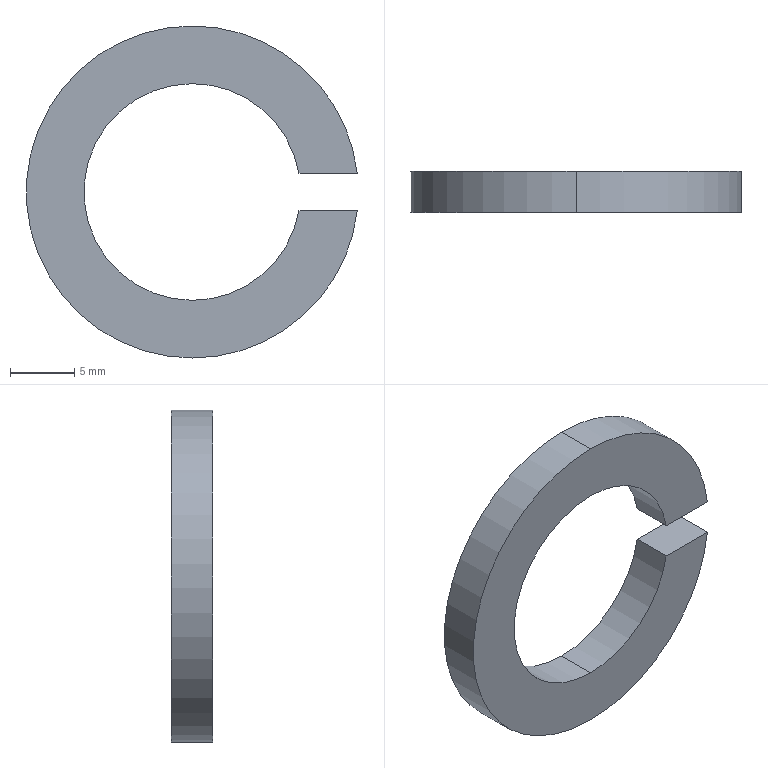Part | SolidWorks | features BaseBody 1 | 1 solid | 10 faces | box 25.819 x 3.2 x 25.9 mm | volume 926.218 mm3 | cylinder 6 | plane 4 | commonest cylinder face diameters 16.9 x3 25.9 x3
STEP:
#1=CARTESIAN_POINT('',(0.,1.6,8.45));
#2=VERTEX_POINT('',#1);
#3=CARTESIAN_POINT('',(0.,1.6,-8.45));
#4=VERTEX_POINT('',#3);
#5=CARTESIAN_POINT('',(0.,1.6,0.));
#6=DIRECTION('',(0.,-1.,0.));
#7=DIRECTION('',(0.,0.,-1.));
#8=AXIS2_PLACEMENT_3D('',#5,#6,#7);
#9=CIRCLE('',#8,8.45);
#10=EDGE_CURVE('',#2,#4,#9,.T.);
#11=ORIENTED_EDGE('',*,*,#10,.F.);
#12=CARTESIAN_POINT('',(0.,-1.6,8.45));
#13=VERTEX_POINT('',#12);
#14=CARTESIAN_POINT('',(0.,0.,8.45));
#15=DIRECTION('',(0.,-1.,0.));
#16=VECTOR('',#15,1000.);
#17=LINE('',#14,#16);
#18=EDGE_CURVE('',#2,#13,#17,.T.);
#19=ORIENTED_EDGE('',*,*,#18,.T.);
#20=CARTESIAN_POINT('',(0.,-1.6,-8.45));
#21=VERTEX_POINT('',#20);
#22=CARTESIAN_POINT('',(0.,-1.6,0.));
#23=DIRECTION('',(0.,-1.,0.));
#24=DIRECTION('',(0.,0.,-1.));
#25=AXIS2_PLACEMENT_3D('',#22,#23,#24);
#26=CIRCLE('',#25,8.45);
#27=EDGE_CURVE('',#13,#21,#26,.T.);
#28=ORIENTED_EDGE('',*,*,#27,.T.);
#29=CARTESIAN_POINT('',(0.,0.,-8.45));
#30=DIRECTION('',(0.,-1.,0.));
#31=VECTOR('',#30,1000.);
#32=LINE('',#29,#31);
#33=EDGE_CURVE('',#4,#21,#32,.T.);
#34=ORIENTED_EDGE('',*,*,#33,.F.);
#35=EDGE_LOOP('',(#11,#19,#28,#34));
#36=FACE_OUTER_BOUND('',#35,.T.);
#37=CARTESIAN_POINT('',(0.,0.,0.));
#38=DIRECTION('',(0.,-1.,0.));
#39=DIRECTION('',(0.,0.,-1.));
#40=AXIS2_PLACEMENT_3D('',#37,#38,#39);
#41=CYLINDRICAL_SURFACE('',#40,8.45);
#42=ADVANCED_FACE('',(#36),#41,.F.);
#43=CARTESIAN_POINT('',(8.325,1.6,-1.45));
#44=VERTEX_POINT('',#43);
#45=CARTESIAN_POINT('',(0.,1.6,0.));
#46=DIRECTION('',(0.,-1.,0.));
#47=DIRECTION('',(0.,0.,-1.));
#48=AXIS2_PLACEMENT_3D('',#45,#46,#47);
#49=CIRCLE('',#48,8.45);
#50=EDGE_CURVE('',#4,#44,#49,.T.);
#51=ORIENTED_EDGE('',*,*,#50,.F.);
#52=ORIENTED_EDGE('',*,*,#33,.T.);
#53=CARTESIAN_POINT('',(8.325,-1.6,-1.45));
#54=VERTEX_POINT('',#53);
#55=CARTESIAN_POINT('',(0.,-1.6,0.));
#56=DIRECTION('',(0.,-1.,0.));
#57=DIRECTION('',(0.,0.,-1.));
#58=AXIS2_PLACEMENT_3D('',#55,#56,#57);
#59=CIRCLE('',#58,8.45);
#60=EDGE_CURVE('',#21,#54,#59,.T.);
#61=ORIENTED_EDGE('',*,*,#60,.T.);
#62=CARTESIAN_POINT('',(8.325,-1.6,-1.45));
#63=DIRECTION('',(0.,1.,0.));
#64=VECTOR('',#63,1000.);
#65=LINE('',#62,#64);
#66=EDGE_CURVE('',#54,#44,#65,.T.);
#67=ORIENTED_EDGE('',*,*,#66,.T.);
#68=EDGE_LOOP('',(#51,#52,#61,#67));
#69=FACE_OUTER_BOUND('',#68,.T.);
#70=CARTESIAN_POINT('',(0.,0.,0.));
#71=DIRECTION('',(0.,-1.,0.));
#72=DIRECTION('',(0.,0.,-1.));
#73=AXIS2_PLACEMENT_3D('',#70,#71,#72);
#74=CYLINDRICAL_SURFACE('',#73,8.45);
#75=ADVANCED_FACE('',(#69),#74,.F.);
#76=CARTESIAN_POINT('',(12.869,1.6,1.45));
#77=VERTEX_POINT('',#76);
#78=CARTESIAN_POINT('',(0.,1.6,12.95));
#79=VERTEX_POINT('',#78);
#80=CARTESIAN_POINT('',(0.,1.6,0.));
#81=DIRECTION('',(0.,-1.,0.));
#82=DIRECTION('',(0.,0.,-1.));
#83=AXIS2_PLACEMENT_3D('',#80,#81,#82);
#84=CIRCLE('',#83,12.95);
#85=EDGE_CURVE('',#77,#79,#84,.T.);
#86=ORIENTED_EDGE('',*,*,#85,.T.);
#87=CARTESIAN_POINT('',(0.,-1.6,12.95));
#88=VERTEX_POINT('',#87);
#89=CARTESIAN_POINT('',(0.,0.,12.95));
#90=DIRECTION('',(0.,-1.,0.));
#91=VECTOR('',#90,1000.);
#92=LINE('',#89,#91);
#93=EDGE_CURVE('',#79,#88,#92,.T.);
#94=ORIENTED_EDGE('',*,*,#93,.T.);
#95=CARTESIAN_POINT('',(12.869,-1.6,1.45));
#96=VERTEX_POINT('',#95);
#97=CARTESIAN_POINT('',(0.,-1.6,0.));
#98=DIRECTION('',(0.,-1.,0.));
#99=DIRECTION('',(0.,0.,-1.));
#100=AXIS2_PLACEMENT_3D('',#97,#98,#99);
#101=CIRCLE('',#100,12.95);
#102=EDGE_CURVE('',#96,#88,#101,.T.);
#103=ORIENTED_EDGE('',*,*,#102,.F.);
#104=CARTESIAN_POINT('',(12.869,0.,1.45));
#105=DIRECTION('',(0.,1.,0.));
#106=VECTOR('',#105,1000.);
#107=LINE('',#104,#106);
#108=EDGE_CURVE('',#96,#77,#107,.T.);
#109=ORIENTED_EDGE('',*,*,#108,.T.);
#110=EDGE_LOOP('',(#86,#94,#103,#109));
#111=FACE_OUTER_BOUND('',#110,.T.);
#112=CARTESIAN_POINT('',(0.,0.,0.));
#113=DIRECTION('',(0.,-1.,0.));
#114=DIRECTION('',(0.,0.,-1.));
#115=AXIS2_PLACEMENT_3D('',#112,#113,#114);
#116=CYLINDRICAL_SURFACE('',#115,12.95);
#117=ADVANCED_FACE('',(#111),#116,.T.);
#118=ORIENTED_EDGE('',*,*,#93,.F.);
#119=CARTESIAN_POINT('',(0.,1.6,-12.95));
#120=VERTEX_POINT('',#119);
#121=CARTESIAN_POINT('',(0.,1.6,0.));
#122=DIRECTION('',(0.,-1.,0.));
#123=DIRECTION('',(0.,0.,-1.));
#124=AXIS2_PLACEMENT_3D('',#121,#122,#123);
#125=CIRCLE('',#124,12.95);
#126=EDGE_CURVE('',#79,#120,#125,.T.);
#127=ORIENTED_EDGE('',*,*,#126,.T.);
#128=CARTESIAN_POINT('',(0.,-1.6,-12.95));
#129=VERTEX_POINT('',#128);
#130=CARTESIAN_POINT('',(0.,0.,-12.95));
#131=DIRECTION('',(0.,-1.,0.));
#132=VECTOR('',#131,1000.);
#133=LINE('',#130,#132);
#134=EDGE_CURVE('',#120,#129,#133,.T.);
#135=ORIENTED_EDGE('',*,*,#134,.T.);
#136=CARTESIAN_POINT('',(0.,-1.6,0.));
#137=DIRECTION('',(0.,-1.,0.));
#138=DIRECTION('',(0.,0.,-1.));
#139=AXIS2_PLACEMENT_3D('',#136,#137,#138);
#140=CIRCLE('',#139,12.95);
#141=EDGE_CURVE('',#88,#129,#140,.T.);
#142=ORIENTED_EDGE('',*,*,#141,.F.);
#143=EDGE_LOOP('',(#118,#127,#135,#142));
#144=FACE_OUTER_BOUND('',#143,.T.);
#145=CARTESIAN_POINT('',(0.,0.,0.));
#146=DIRECTION('',(0.,-1.,0.));
#147=DIRECTION('',(0.,0.,-1.));
#148=AXIS2_PLACEMENT_3D('',#145,#146,#147);
#149=CYLINDRICAL_SURFACE('',#148,12.95);
#150=ADVANCED_FACE('',(#144),#149,.T.);
#151=ORIENTED_EDGE('',*,*,#134,.F.);
#152=CARTESIAN_POINT('',(12.869,1.6,-1.45));
#153=VERTEX_POINT('',#152);
#154=CARTESIAN_POINT('',(0.,1.6,0.));
#155=DIRECTION('',(0.,-1.,0.));
#156=DIRECTION('',(0.,0.,-1.));
#157=AXIS2_PLACEMENT_3D('',#154,#155,#156);
#158=CIRCLE('',#157,12.95);
#159=EDGE_CURVE('',#120,#153,#158,.T.);
#160=ORIENTED_EDGE('',*,*,#159,.T.);
#161=CARTESIAN_POINT('',(12.869,-1.6,-1.45));
#162=VERTEX_POINT('',#161);
#163=CARTESIAN_POINT('',(12.869,0.,-1.45));
#164=DIRECTION('',(0.,-1.,0.));
#165=VECTOR('',#164,1000.);
#166=LINE('',#163,#165);
#167=EDGE_CURVE('',#153,#162,#166,.T.);
#168=ORIENTED_EDGE('',*,*,#167,.T.);
#169=CARTESIAN_POINT('',(0.,-1.6,0.));
#170=DIRECTION('',(0.,-1.,0.));
#171=DIRECTION('',(0.,0.,-1.));
#172=AXIS2_PLACEMENT_3D('',#169,#170,#171);
#173=CIRCLE('',#172,12.95);
#174=EDGE_CURVE('',#129,#162,#173,.T.);
#175=ORIENTED_EDGE('',*,*,#174,.F.);
#176=EDGE_LOOP('',(#151,#160,#168,#175));
#177=FACE_OUTER_BOUND('',#176,.T.);
#178=CARTESIAN_POINT('',(0.,0.,0.));
#179=DIRECTION('',(0.,-1.,0.));
#180=DIRECTION('',(0.,0.,-1.));
#181=AXIS2_PLACEMENT_3D('',#178,#179,#180);
#182=CYLINDRICAL_SURFACE('',#181,12.95);
#183=ADVANCED_FACE('',(#177),#182,.T.);
#184=CARTESIAN_POINT('',(8.325,1.6,1.45));
#185=VERTEX_POINT('',#184);
#186=CARTESIAN_POINT('',(0.,1.6,0.));
#187=DIRECTION('',(0.,-1.,0.));
#188=DIRECTION('',(0.,0.,-1.));
#189=AXIS2_PLACEMENT_3D('',#186,#187,#188);
#190=CIRCLE('',#189,8.45);
#191=EDGE_CURVE('',#185,#2,#190,.T.);
#192=ORIENTED_EDGE('',*,*,#191,.T.);
#193=ORIENTED_EDGE('',*,*,#10,.T.);
#194=ORIENTED_EDGE('',*,*,#50,.T.);
#195=CARTESIAN_POINT('',(8.325,1.6,-1.45));
#196=DIRECTION('',(-1.,0.,0.));
#197=VECTOR('',#196,1000.);
#198=LINE('',#195,#197);
#199=EDGE_CURVE('',#153,#44,#198,.T.);
#200=ORIENTED_EDGE('',*,*,#199,.F.);
#201=ORIENTED_EDGE('',*,*,#159,.F.);
#202=ORIENTED_EDGE('',*,*,#126,.F.);
#203=ORIENTED_EDGE('',*,*,#85,.F.);
#204=CARTESIAN_POINT('',(8.325,1.6,1.45));
#205=DIRECTION('',(1.,0.,0.));
#206=VECTOR('',#205,1000.);
#207=LINE('',#204,#206);
#208=EDGE_CURVE('',#185,#77,#207,.T.);
#209=ORIENTED_EDGE('',*,*,#208,.F.);
#210=EDGE_LOOP('',(#192,#193,#194,#200,#201,#202,#203,#209));
#211=FACE_OUTER_BOUND('',#210,.T.);
#212=CARTESIAN_POINT('',(0.,1.6,0.));
#213=DIRECTION('',(0.,-1.,0.));
#214=DIRECTION('',(0.,0.,-1.));
#215=AXIS2_PLACEMENT_3D('',#212,#213,#214);
#216=PLANE('',#215);
#217=ADVANCED_FACE('',(#211),#216,.F.);
#218=ORIENTED_EDGE('',*,*,#18,.F.);
#219=ORIENTED_EDGE('',*,*,#191,.F.);
#220=CARTESIAN_POINT('',(8.325,-1.6,1.45));
#221=VERTEX_POINT('',#220);
#222=CARTESIAN_POINT('',(8.325,-1.6,1.45));
#223=DIRECTION('',(0.,1.,0.));
#224=VECTOR('',#223,1000.);
#225=LINE('',#222,#224);
#226=EDGE_CURVE('',#221,#185,#225,.T.);
#227=ORIENTED_EDGE('',*,*,#226,.F.);
#228=CARTESIAN_POINT('',(0.,-1.6,0.));
#229=DIRECTION('',(0.,-1.,0.));
#230=DIRECTION('',(0.,0.,-1.));
#231=AXIS2_PLACEMENT_3D('',#228,#229,#230);
#232=CIRCLE('',#231,8.45);
#233=EDGE_CURVE('',#221,#13,#232,.T.);
#234=ORIENTED_EDGE('',*,*,#233,.T.);
#235=EDGE_LOOP('',(#218,#219,#227,#234));
#236=FACE_OUTER_BOUND('',#235,.T.);
#237=CARTESIAN_POINT('',(0.,0.,0.));
#238=DIRECTION('',(0.,-1.,0.));
#239=DIRECTION('',(0.,0.,-1.));
#240=AXIS2_PLACEMENT_3D('',#237,#238,#239);
#241=CYLINDRICAL_SURFACE('',#240,8.45);
#242=ADVANCED_FACE('',(#236),#241,.F.);
#243=CARTESIAN_POINT('',(0.,-1.6,-1.45));
#244=DIRECTION('',(1.,0.,0.));
#245=VECTOR('',#244,1000.);
#246=LINE('',#243,#245);
#247=EDGE_CURVE('',#54,#162,#246,.T.);
#248=ORIENTED_EDGE('',*,*,#247,.F.);
#249=ORIENTED_EDGE('',*,*,#60,.F.);
#250=ORIENTED_EDGE('',*,*,#27,.F.);
#251=ORIENTED_EDGE('',*,*,#233,.F.);
#252=CARTESIAN_POINT('',(8.325,-1.6,1.45));
#253=DIRECTION('',(1.,0.,0.));
#254=VECTOR('',#253,1000.);
#255=LINE('',#252,#254);
#256=EDGE_CURVE('',#221,#96,#255,.T.);
#257=ORIENTED_EDGE('',*,*,#256,.T.);
#258=ORIENTED_EDGE('',*,*,#102,.T.);
#259=ORIENTED_EDGE('',*,*,#141,.T.);
#260=ORIENTED_EDGE('',*,*,#174,.T.);
#261=EDGE_LOOP('',(#248,#249,#250,#251,#257,#258,#259,#260));
#262=FACE_OUTER_BOUND('',#261,.T.);
#263=CARTESIAN_POINT('',(0.,-1.6,0.));
#264=DIRECTION('',(0.,-1.,0.));
#265=DIRECTION('',(0.,0.,-1.));
#266=AXIS2_PLACEMENT_3D('',#263,#264,#265);
#267=PLANE('',#266);
#268=ADVANCED_FACE('',(#262),#267,.T.);
#269=ORIENTED_EDGE('',*,*,#256,.F.);
#270=ORIENTED_EDGE('',*,*,#226,.T.);
#271=ORIENTED_EDGE('',*,*,#208,.T.);
#272=ORIENTED_EDGE('',*,*,#108,.F.);
#273=EDGE_LOOP('',(#269,#270,#271,#272));
#274=FACE_OUTER_BOUND('',#273,.T.);
#275=CARTESIAN_POINT('',(8.325,-1.6,1.45));
#276=DIRECTION('',(0.,0.,1.));
#277=DIRECTION('',(1.,0.,0.));
#278=AXIS2_PLACEMENT_3D('',#275,#276,#277);
#279=PLANE('',#278);
#280=ADVANCED_FACE('',(#274),#279,.F.);
#281=ORIENTED_EDGE('',*,*,#199,.T.);
#282=ORIENTED_EDGE('',*,*,#66,.F.);
#283=ORIENTED_EDGE('',*,*,#247,.T.);
#284=ORIENTED_EDGE('',*,*,#167,.F.);
#285=EDGE_LOOP('',(#281,#282,#283,#284));
#286=FACE_OUTER_BOUND('',#285,.T.);
#287=CARTESIAN_POINT('',(8.325,-1.6,-1.45));
#288=DIRECTION('',(0.,0.,-1.));
#289=DIRECTION('',(-1.,0.,0.));
#290=AXIS2_PLACEMENT_3D('',#287,#288,#289);
#291=PLANE('',#290);
#292=ADVANCED_FACE('',(#286),#291,.F.);
#293=CLOSED_SHELL('',(#42,#75,#117,#150,#183,#217,#242,#268,#280,#292));
#294=MANIFOLD_SOLID_BREP('',#293);
#295=CARTESIAN_POINT('',(0.,0.,0.));
#296=DIRECTION('',(0.,0.,1.));
#297=DIRECTION('',(1.,0.,0.));
#298=AXIS2_PLACEMENT_3D('',#295,#296,#297);
#299=(LENGTH_UNIT()NAMED_UNIT(*)SI_UNIT(.MILLI.,.METRE.));
#300=UNCERTAINTY_MEASURE_WITH_UNIT(LENGTH_MEASURE(0.00001),#299,'','');
#301=(NAMED_UNIT(*)PLANE_ANGLE_UNIT()SI_UNIT($,.RADIAN.));
#302=(NAMED_UNIT(*)SI_UNIT($,.STERADIAN.)SOLID_ANGLE_UNIT());
#303=(GEOMETRIC_REPRESENTATION_CONTEXT(3)GLOBAL_UNCERTAINTY_ASSIGNED_CONTEXT((#300))GLOBAL_UNIT_ASSIGNED_CONTEXT((#299,#301,#302))REPRESENTATION_CONTEXT('',''));
#304=ADVANCED_BREP_SHAPE_REPRESENTATION('',(#294,#298),#303);